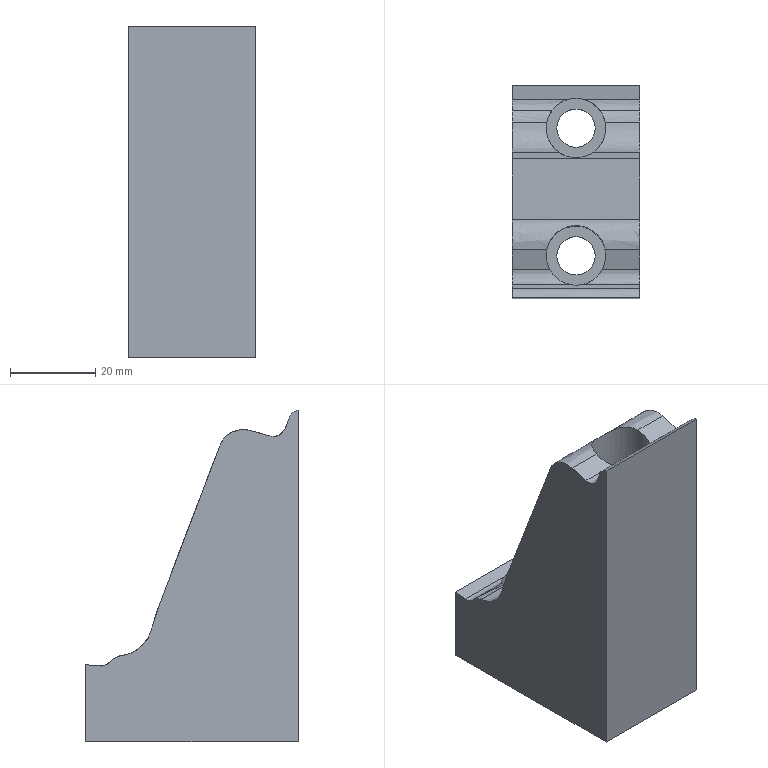Part | NX | features solid 2 | 1 solid | 29 faces | box 30 x 50 x 77.929 mm | volume 60557 mm3 | spline 18 | plane 7 | cylinder 4 | commonest cylinder face diameters 9 x2 14 x2